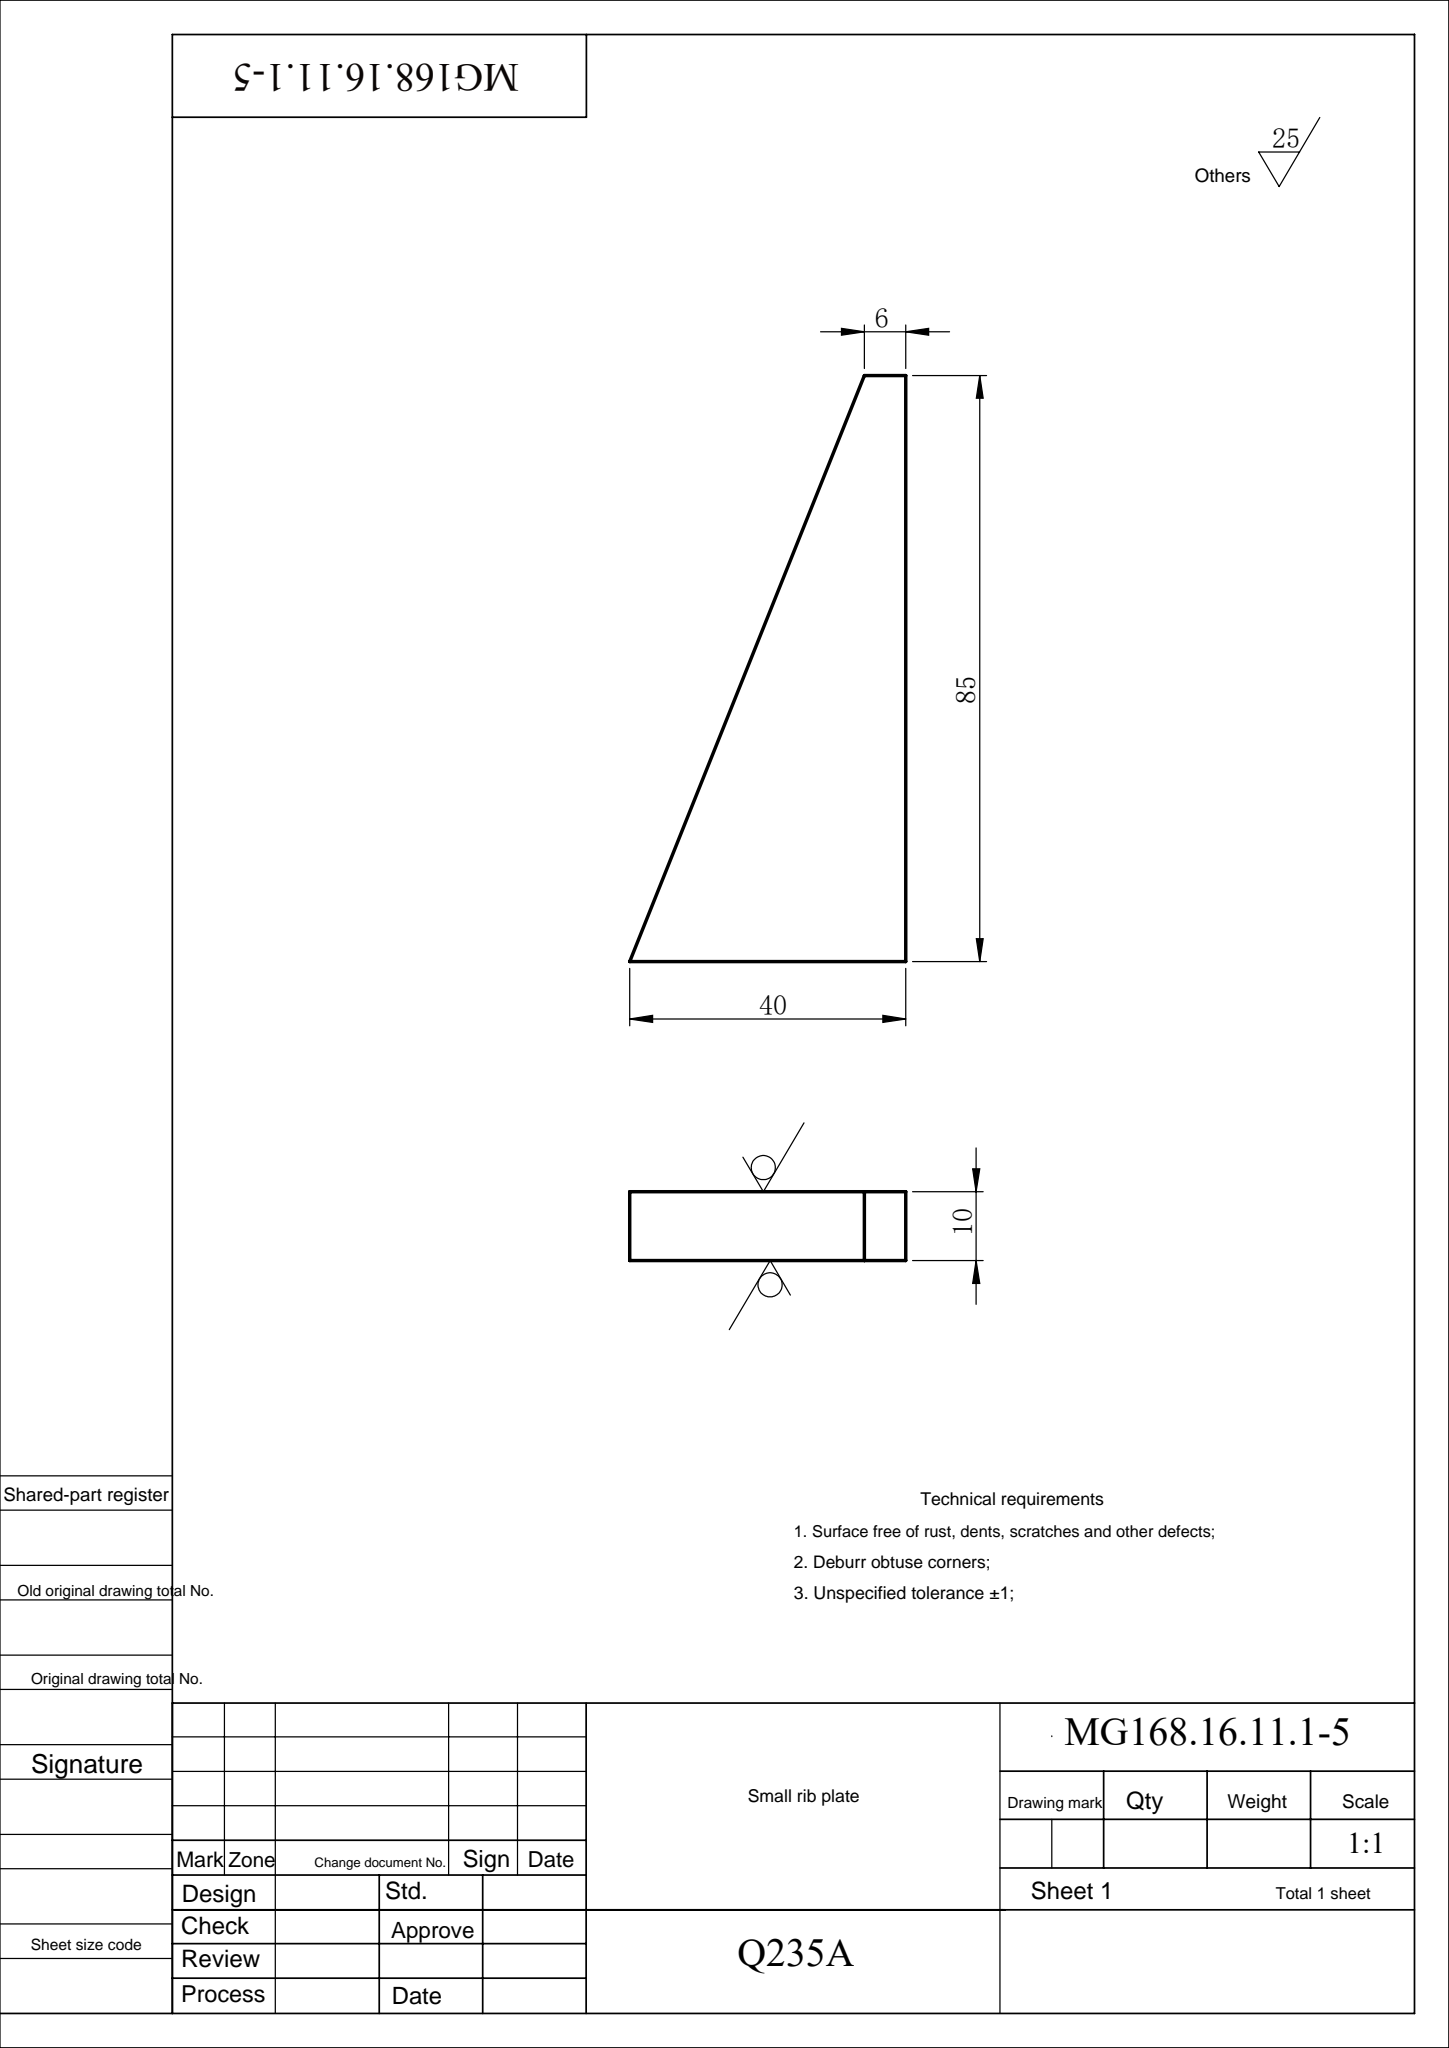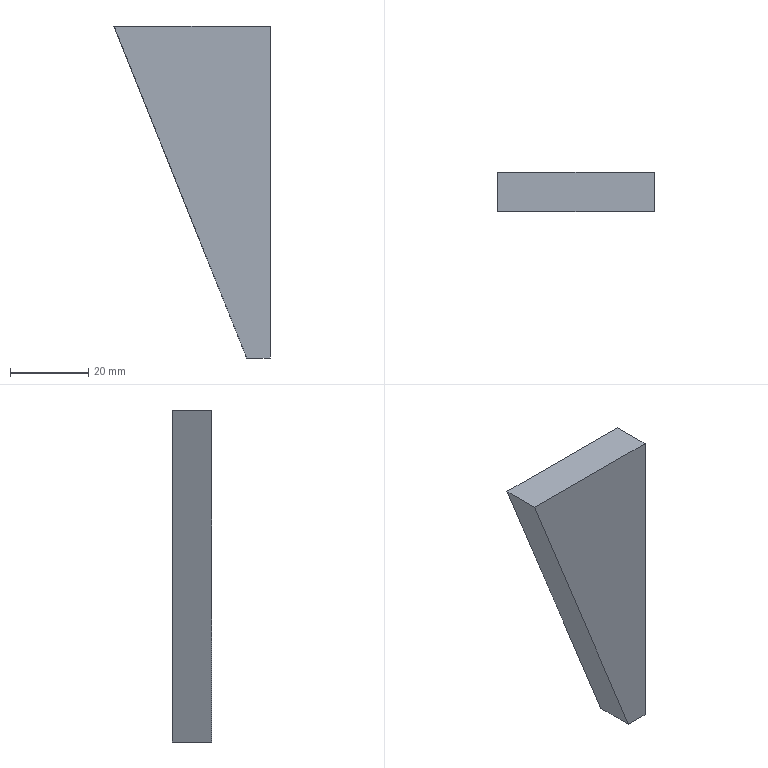Part | SolidWorks | features Extrusion 1 | 1 solid | 6 faces | box 40 x 10 x 85 mm | volume 19550 mm3 | plane 6
STEP:
#1=CARTESIAN_POINT('',(0.,-5.,0.));
#2=VERTEX_POINT('',#1);
#3=CARTESIAN_POINT('',(0.,-5.,-85.));
#4=VERTEX_POINT('',#3);
#5=CARTESIAN_POINT('',(0.,-5.,0.));
#6=DIRECTION('',(0.,0.,-1.));
#7=VECTOR('',#6,1000.);
#8=LINE('',#5,#7);
#9=EDGE_CURVE('',#2,#4,#8,.T.);
#10=ORIENTED_EDGE('',*,*,#9,.T.);
#11=CARTESIAN_POINT('',(0.,5.,-85.));
#12=VERTEX_POINT('',#11);
#13=CARTESIAN_POINT('',(0.,5.,-85.));
#14=DIRECTION('',(0.,-1.,0.));
#15=VECTOR('',#14,1000.);
#16=LINE('',#13,#15);
#17=EDGE_CURVE('',#12,#4,#16,.T.);
#18=ORIENTED_EDGE('',*,*,#17,.F.);
#19=CARTESIAN_POINT('',(0.,5.,0.));
#20=VERTEX_POINT('',#19);
#21=CARTESIAN_POINT('',(0.,5.,0.));
#22=DIRECTION('',(0.,0.,-1.));
#23=VECTOR('',#22,1000.);
#24=LINE('',#21,#23);
#25=EDGE_CURVE('',#20,#12,#24,.T.);
#26=ORIENTED_EDGE('',*,*,#25,.F.);
#27=CARTESIAN_POINT('',(0.,5.,0.));
#28=DIRECTION('',(0.,-1.,0.));
#29=VECTOR('',#28,1000.);
#30=LINE('',#27,#29);
#31=EDGE_CURVE('',#20,#2,#30,.T.);
#32=ORIENTED_EDGE('',*,*,#31,.T.);
#33=EDGE_LOOP('',(#10,#18,#26,#32));
#34=FACE_OUTER_BOUND('',#33,.T.);
#35=CARTESIAN_POINT('',(0.,5.,0.));
#36=DIRECTION('',(-1.,0.,0.));
#37=DIRECTION('',(0.,0.,1.));
#38=AXIS2_PLACEMENT_3D('',#35,#36,#37);
#39=PLANE('',#38);
#40=ADVANCED_FACE('',(#34),#39,.F.);
#41=CARTESIAN_POINT('',(-6.,-5.,-85.));
#42=VERTEX_POINT('',#41);
#43=CARTESIAN_POINT('',(0.,-5.,-85.));
#44=DIRECTION('',(-1.,0.,0.));
#45=VECTOR('',#44,1000.);
#46=LINE('',#43,#45);
#47=EDGE_CURVE('',#4,#42,#46,.T.);
#48=ORIENTED_EDGE('',*,*,#47,.T.);
#49=CARTESIAN_POINT('',(-6.,5.,-85.));
#50=VERTEX_POINT('',#49);
#51=CARTESIAN_POINT('',(-6.,5.,-85.));
#52=DIRECTION('',(0.,-1.,0.));
#53=VECTOR('',#52,1000.);
#54=LINE('',#51,#53);
#55=EDGE_CURVE('',#50,#42,#54,.T.);
#56=ORIENTED_EDGE('',*,*,#55,.F.);
#57=CARTESIAN_POINT('',(0.,5.,-85.));
#58=DIRECTION('',(-1.,0.,0.));
#59=VECTOR('',#58,1000.);
#60=LINE('',#57,#59);
#61=EDGE_CURVE('',#12,#50,#60,.T.);
#62=ORIENTED_EDGE('',*,*,#61,.F.);
#63=ORIENTED_EDGE('',*,*,#17,.T.);
#64=EDGE_LOOP('',(#48,#56,#62,#63));
#65=FACE_OUTER_BOUND('',#64,.T.);
#66=CARTESIAN_POINT('',(0.,5.,-85.));
#67=DIRECTION('',(0.,0.,1.));
#68=DIRECTION('',(1.,0.,0.));
#69=AXIS2_PLACEMENT_3D('',#66,#67,#68);
#70=PLANE('',#69);
#71=ADVANCED_FACE('',(#65),#70,.F.);
#72=CARTESIAN_POINT('',(-40.,-5.,0.));
#73=VERTEX_POINT('',#72);
#74=CARTESIAN_POINT('',(-6.,-5.,-85.));
#75=DIRECTION('',(-0.3714,0.,0.9285));
#76=VECTOR('',#75,1000.);
#77=LINE('',#74,#76);
#78=EDGE_CURVE('',#42,#73,#77,.T.);
#79=ORIENTED_EDGE('',*,*,#78,.T.);
#80=CARTESIAN_POINT('',(-40.,5.,0.));
#81=VERTEX_POINT('',#80);
#82=CARTESIAN_POINT('',(-40.,5.,0.));
#83=DIRECTION('',(0.,-1.,0.));
#84=VECTOR('',#83,1000.);
#85=LINE('',#82,#84);
#86=EDGE_CURVE('',#81,#73,#85,.T.);
#87=ORIENTED_EDGE('',*,*,#86,.F.);
#88=CARTESIAN_POINT('',(-6.,5.,-85.));
#89=DIRECTION('',(-0.3714,0.,0.9285));
#90=VECTOR('',#89,1000.);
#91=LINE('',#88,#90);
#92=EDGE_CURVE('',#50,#81,#91,.T.);
#93=ORIENTED_EDGE('',*,*,#92,.F.);
#94=ORIENTED_EDGE('',*,*,#55,.T.);
#95=EDGE_LOOP('',(#79,#87,#93,#94));
#96=FACE_OUTER_BOUND('',#95,.T.);
#97=CARTESIAN_POINT('',(-6.,5.,-85.));
#98=DIRECTION('',(0.9285,0.,0.3714));
#99=DIRECTION('',(0.3714,0.,-0.9285));
#100=AXIS2_PLACEMENT_3D('',#97,#98,#99);
#101=PLANE('',#100);
#102=ADVANCED_FACE('',(#96),#101,.F.);
#103=CARTESIAN_POINT('',(0.,-5.,0.));
#104=DIRECTION('',(1.,0.,0.));
#105=VECTOR('',#104,1000.);
#106=LINE('',#103,#105);
#107=EDGE_CURVE('',#73,#2,#106,.T.);
#108=ORIENTED_EDGE('',*,*,#107,.T.);
#109=ORIENTED_EDGE('',*,*,#31,.F.);
#110=CARTESIAN_POINT('',(0.,5.,0.));
#111=DIRECTION('',(1.,0.,0.));
#112=VECTOR('',#111,1000.);
#113=LINE('',#110,#112);
#114=EDGE_CURVE('',#81,#20,#113,.T.);
#115=ORIENTED_EDGE('',*,*,#114,.F.);
#116=ORIENTED_EDGE('',*,*,#86,.T.);
#117=EDGE_LOOP('',(#108,#109,#115,#116));
#118=FACE_OUTER_BOUND('',#117,.T.);
#119=CARTESIAN_POINT('',(0.,5.,0.));
#120=DIRECTION('',(0.,0.,-1.));
#121=DIRECTION('',(-1.,0.,0.));
#122=AXIS2_PLACEMENT_3D('',#119,#120,#121);
#123=PLANE('',#122);
#124=ADVANCED_FACE('',(#118),#123,.F.);
#125=ORIENTED_EDGE('',*,*,#25,.T.);
#126=ORIENTED_EDGE('',*,*,#61,.T.);
#127=ORIENTED_EDGE('',*,*,#92,.T.);
#128=ORIENTED_EDGE('',*,*,#114,.T.);
#129=EDGE_LOOP('',(#125,#126,#127,#128));
#130=FACE_OUTER_BOUND('',#129,.T.);
#131=CARTESIAN_POINT('',(0.,5.,0.));
#132=DIRECTION('',(0.,1.,0.));
#133=DIRECTION('',(0.,0.,1.));
#134=AXIS2_PLACEMENT_3D('',#131,#132,#133);
#135=PLANE('',#134);
#136=ADVANCED_FACE('',(#130),#135,.T.);
#137=ORIENTED_EDGE('',*,*,#9,.F.);
#138=ORIENTED_EDGE('',*,*,#107,.F.);
#139=ORIENTED_EDGE('',*,*,#78,.F.);
#140=ORIENTED_EDGE('',*,*,#47,.F.);
#141=EDGE_LOOP('',(#137,#138,#139,#140));
#142=FACE_OUTER_BOUND('',#141,.T.);
#143=CARTESIAN_POINT('',(0.,-5.,0.));
#144=DIRECTION('',(0.,1.,0.));
#145=DIRECTION('',(0.,0.,1.));
#146=AXIS2_PLACEMENT_3D('',#143,#144,#145);
#147=PLANE('',#146);
#148=ADVANCED_FACE('',(#142),#147,.F.);
#149=CLOSED_SHELL('',(#40,#71,#102,#124,#136,#148));
#150=MANIFOLD_SOLID_BREP('',#149);
#151=CARTESIAN_POINT('',(0.,0.,0.));
#152=DIRECTION('',(0.,0.,1.));
#153=DIRECTION('',(1.,0.,0.));
#154=AXIS2_PLACEMENT_3D('',#151,#152,#153);
#155=(LENGTH_UNIT()NAMED_UNIT(*)SI_UNIT(.MILLI.,.METRE.));
#156=UNCERTAINTY_MEASURE_WITH_UNIT(LENGTH_MEASURE(0.00001),#155,'','');
#157=(NAMED_UNIT(*)PLANE_ANGLE_UNIT()SI_UNIT($,.RADIAN.));
#158=(NAMED_UNIT(*)SI_UNIT($,.STERADIAN.)SOLID_ANGLE_UNIT());
#159=(GEOMETRIC_REPRESENTATION_CONTEXT(3)GLOBAL_UNCERTAINTY_ASSIGNED_CONTEXT((#156))GLOBAL_UNIT_ASSIGNED_CONTEXT((#155,#157,#158))REPRESENTATION_CONTEXT('',''));
#160=ADVANCED_BREP_SHAPE_REPRESENTATION('',(#150,#154),#159);